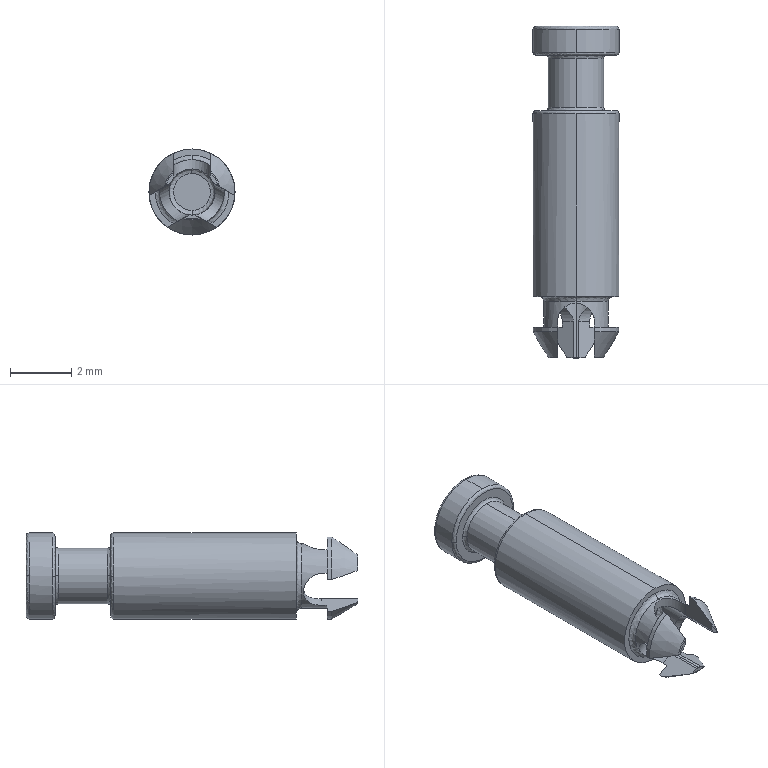Part | SolidWorks | features BaseBody 1 | 1 solid | 54 faces | box 2.8 x 10.8 x 2.8 mm | volume 49.198 mm3 | plane 17 | spline 17 | cylinder 17 | cone 3 | commonest cylinder face diameters 2.8 x8 1.2 x3 1.5 x2 1.8 x2 2.1 x2